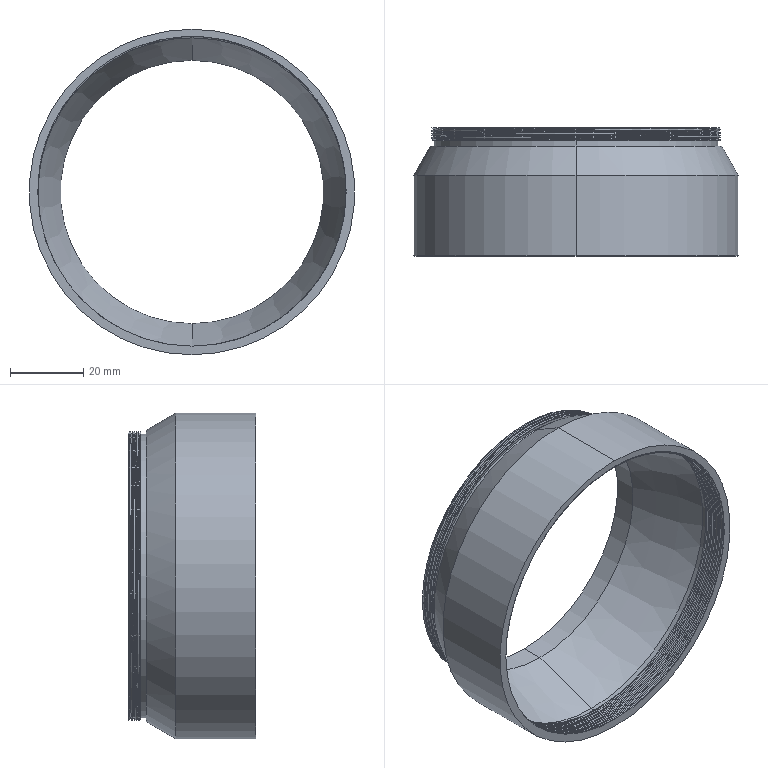Part | NX | features BREP 1 | 1 solid | 48 faces | box 89 x 35 x 89 mm | volume 31154 mm3 | cylinder 35 | plane 5 | cone 4 | spline 4 | commonest cylinder face diameters 84.3 x16 79 x9 72 x2 77.5 x2 86 x2 89 x2